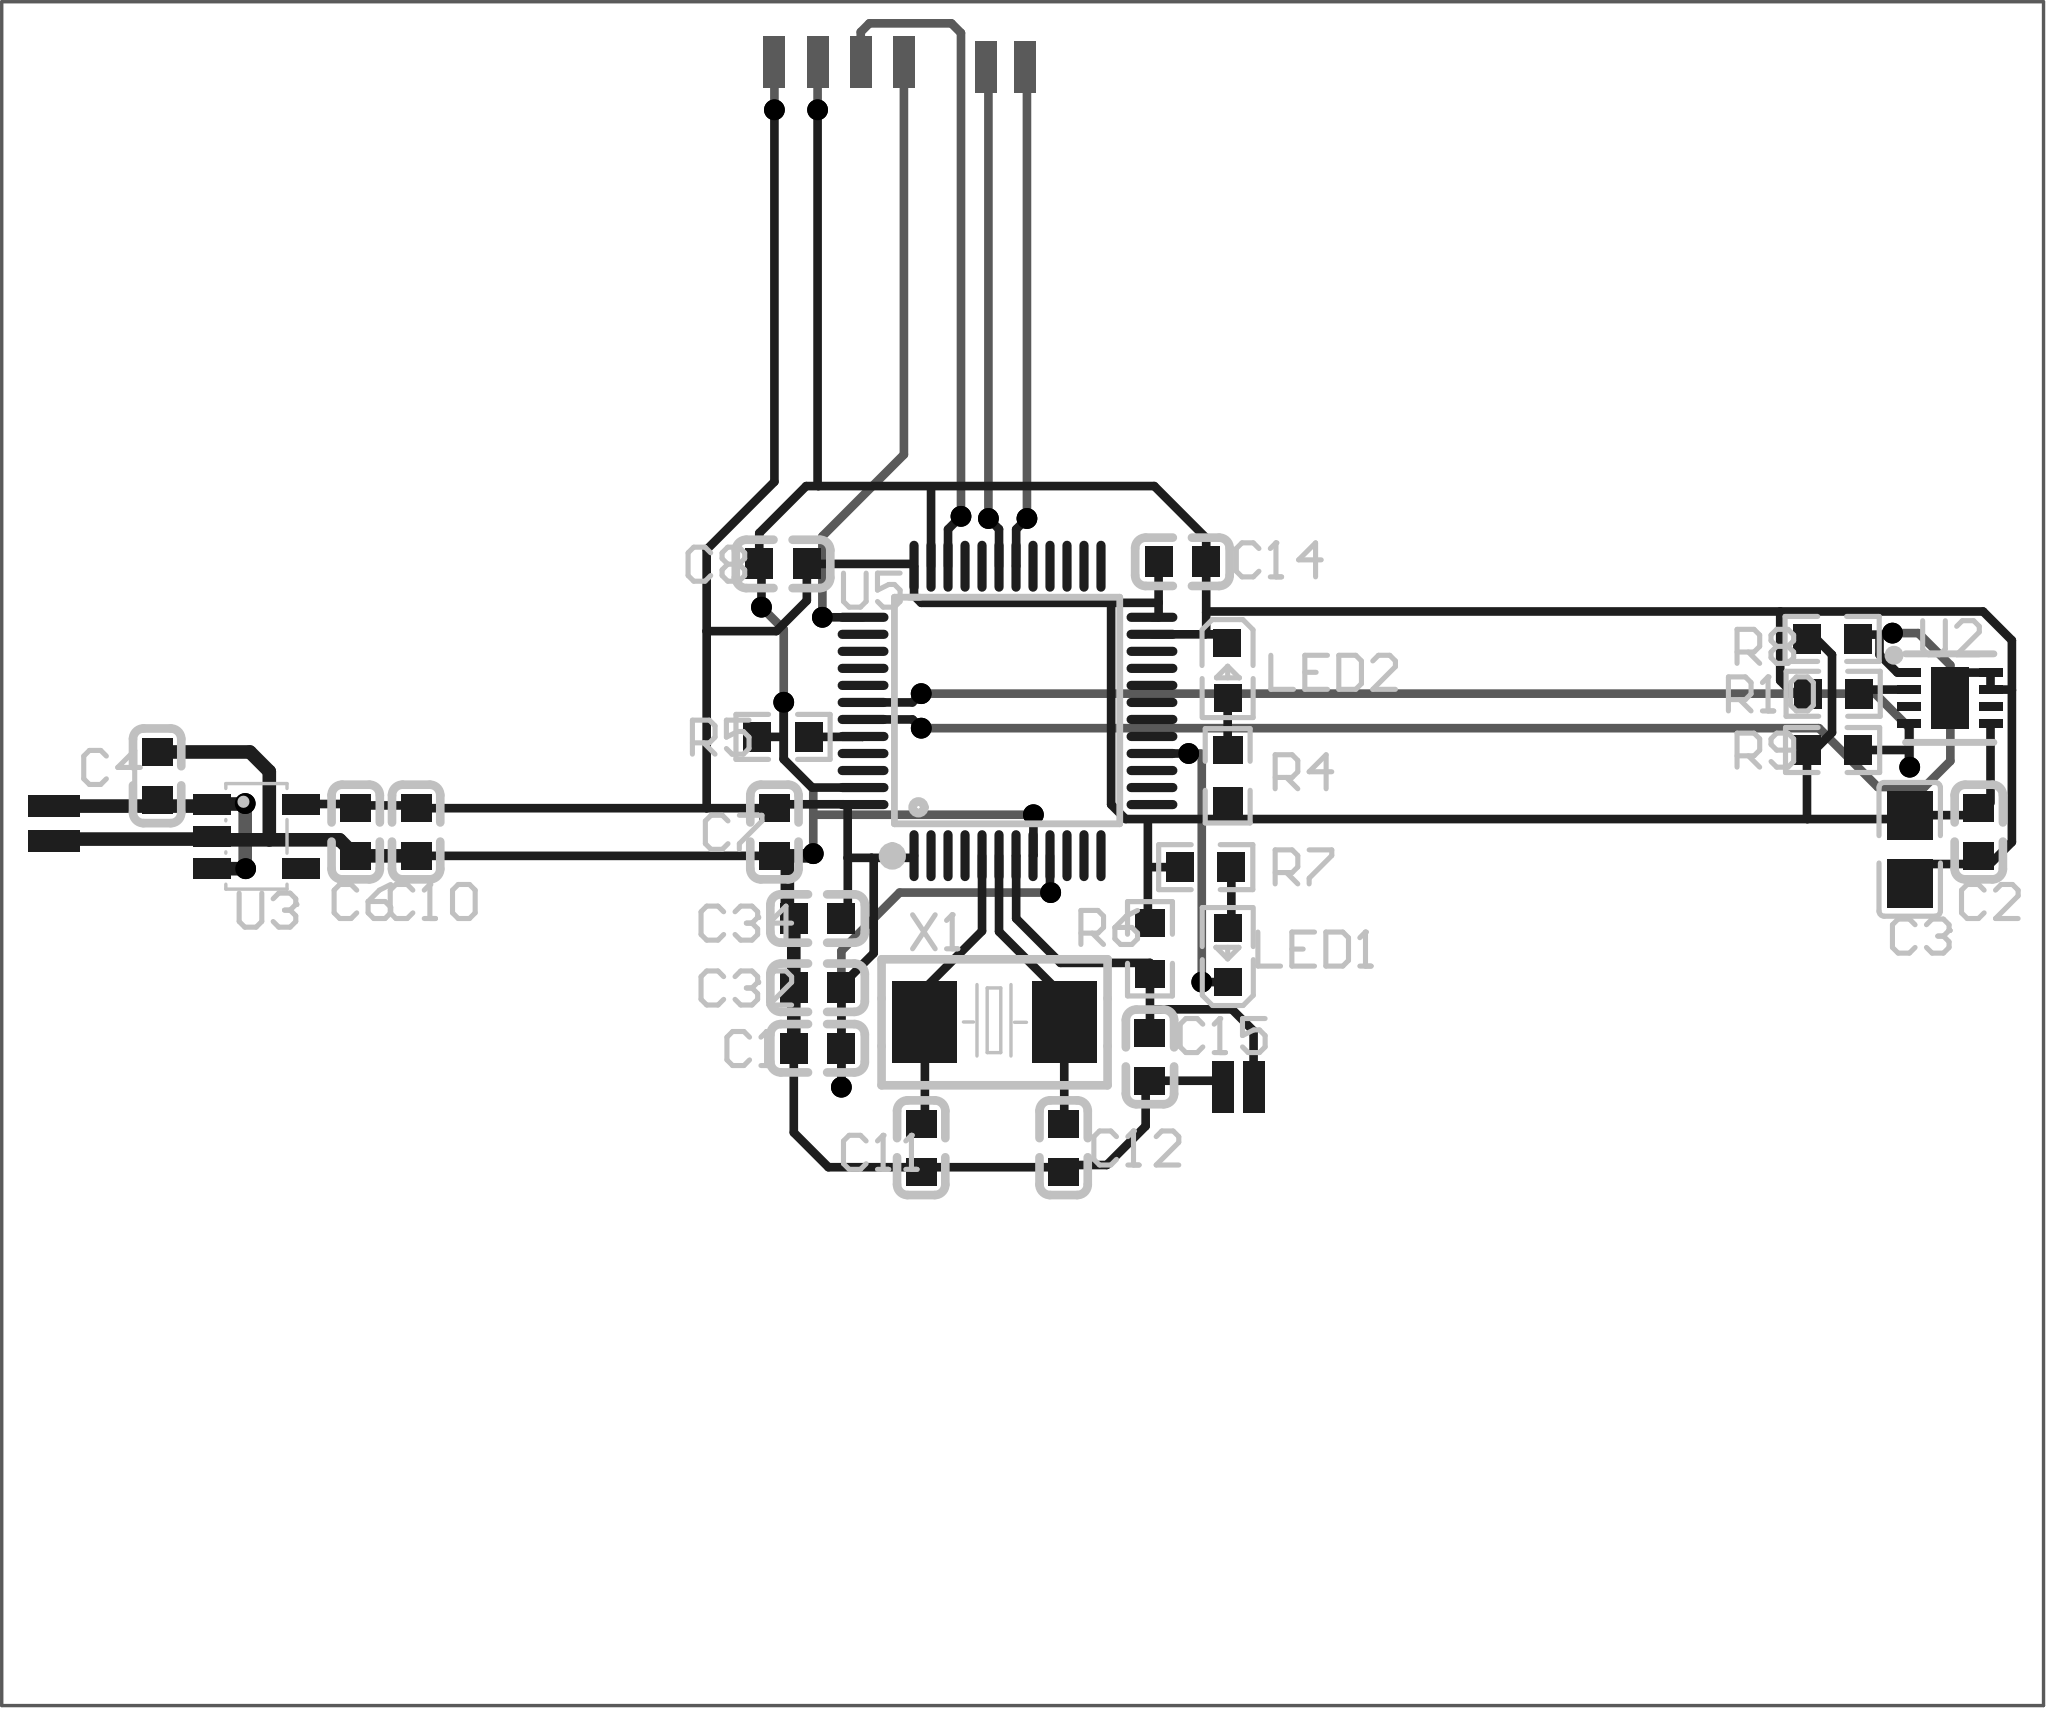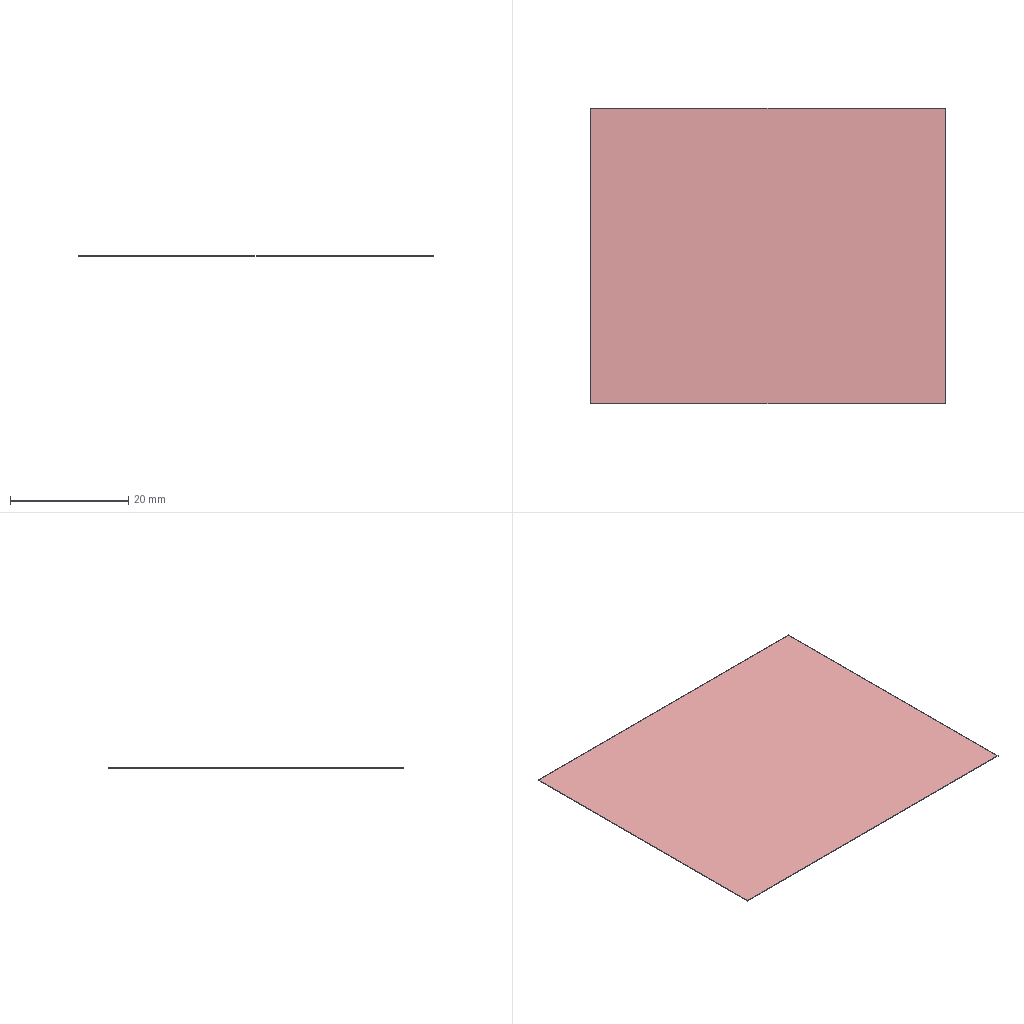Circuit board layout | Altium Designer | box 60.1 x 50 x 0.1 mm
Layer stack:
# Altium Designer layer stack of  (unit mm; dielectric type: 0 none, 1 core, 2 prepreg, 3 surface material)
index,name,kind,layer,copper_thickness_mm,dielectric_type,dielectric_thickness_mm,dielectric_material,dielectric_constant
0,Top Paste Mask Layer,other,,,,,,
1,Top Silkscreen Layer,other,,,,,,
2,Top Solder Mask Layer,dielectric,,,3,0.027,,3.3
3,Top Layer,copper,Top Layer,0.012,,,,
4,Dielectric1,dielectric,,,3,0.025,FR4,4.5
5,Bottom Layer,copper,Bottom Layer,0.012,,,,
6,Bottom Solder Mask Layer,dielectric,,,3,0.027,,3.3
7,Bottom Silkscreen Layer,other,,,,,,
8,Bottom Paste Mask Layer,other,,,,,,
# drill layer pairs: low layer,high layer
drill_pair,Top Layer,Bottom Layer
Part placement:
Designator,Comment,Layer,Footprint,Center-X(mm),Center-Y(mm),Rotation
C7,100nF,TopLayer,C0603,98.933,101.854,90
C8,100nF,TopLayer,C0603,99.187,109.728,180
C14,100nF,TopLayer,C0603,110.936,109.79,0
C15,100nF,TopLayer,C0603,109.982,95.25,270
C32,100nF,TopLayer,C0603,100.203,97.282,0
C34,100nF,TopLayer,C0603,100.203,99.314,180
LED2,,TopLayer,LED_0603,112.26,106.604,270
R4,1K,TopLayer,R0603,112.268,103.505,90
R5,10K,TopLayer,R0603,99.187,104.648,180
R6,10K,TopLayer,R0603,109.982,98.425,90
U5,STM32F103C8T6,TopLayer,LQFP-48_L7.0-W7.0-P0.50-LS9.0-BL,105.791,105.41,0
C2,100nF,TopLayer,C0603,134.366,101.854,270
C3,4.7uF,TopLayer,C0805,132.334,101.346,90
C4,10uF,TopLayer,C0603,80.772,103.505,270
C6,10uF,TopLayer,C0603,86.614,101.854,270
C10,100nF,TopLayer,C0603,88.392,101.854,90
LED1,,TopLayer,LED_0603,112.276,98.247,90
R7,1K,TopLayer,R0603,111.623,100.823,0
R8,10K,TopLayer,R0603,130.052,107.525,180
R9,10K,TopLayer,R0603,130.065,104.263,180
R10,10K,TopLayer,R0603,130.082,105.914,180
U2,SHT30-DIS-B2.5KS,TopLayer,DFN-8_L2.5-W2.5-P0.50-BL-EP,133.511,105.787,270
U3,TLV75533PDBVR,TopLayer,SOT-23-5_L3.0-W1.7-P0.95-LS2.8-BR,83.693,101.727,180
X1,8MHz,TopLayer,CRYSTAL-SMD_L5.0-W3.2,105.41,96.266,180
C11,20pF,TopLayer,C0603,103.251,92.583,90
C12,20pF,TopLayer,C0603,107.442,92.583,90
C1,1uF,TopLayer,C0603,100.203,95.504,0
Pad and via stacks:
# Altium Designer via and pad stacks of  (unit mm). Each distinct definition once, with the count of objects using it.
# via: kind,start_layer,end_layer,hole_mm,diameter_mm,mode(0 simple;1 top-mid-bottom;2 full stack),diameter_per_layer,count,example_net
# pad: kind,layer,hole_mm,hole_type(0 round;1 square;2 slot),plating,top_size,top_shape(1 round;2 rect;3 octagon;9 rounded rect),mid_size,bottom_size,mode,footprint,size_per_layer,count,example
pad,Top Layer,0,0,plated,0.8x0.9,2,0.8x0.9,0.8x0.9,0,C0603,,26,C7.2
pad,Top Layer,0,0,plated,0.8001x0.8001,2,0.8001x0.8001,0.8001x0.8001,0,LED_0603,,4,LED2.1
pad,Top Layer,0,0,plated,0.8065x0.864,2,0.8065x0.864,0.8065x0.864,0,R0603,,14,R4.2
pad,Top Layer,0,0,plated,0.27x1.5,1,0.27x1.5,0.27x1.5,0,LQFP-48_L7.0-W7.0-P0.50-LS9.0-BL,,24,U5.1
pad,Top Layer,0,0,plated,1.5x0.27,1,1.5x0.27,1.5x0.27,0,LQFP-48_L7.0-W7.0-P0.50-LS9.0-BL,,24,U5.13
pad,Top Layer,0,0,plated,1.41x1.35,2,1.41x1.35,1.41x1.35,0,C0805,,2,C3.2
pad,Top Layer,0,0,plated,1.8x1.1,2,1.8x1.1,1.8x1.1,0,DFN-8_L2.5-W2.5-P0.50-BL-EP,,1,U2.9
pad,Top Layer,0,0,plated,0.25x0.7,2,0.25x0.7,0.25x0.7,0,DFN-8_L2.5-W2.5-P0.50-BL-EP,,8,U2.5
pad,Top Layer,0,0,plated,1.1x0.6,2,1.1x0.6,1.1x0.6,0,SOT-23-5_L3.0-W1.7-P0.95-LS2.8-BR,,5,U3.5
pad,Top Layer,0,0,plated,1.524x0.635,2,1.524x0.635,1.524x0.635,0,,,4,4
pad,Top Layer,0,0,plated,1.9x2.4,2,1.9x2.4,1.9x2.4,0,CRYSTAL-SMD_L5.0-W3.2,,2,X1.2
pad,Bottom Layer,0,0,plated,1.524x0.635,2,1.524x0.635,1.524x0.635,0,,,6,1
via,Top Layer,Bottom Layer,0.3048,0.61,0,,20,GND
Design rules, without the lines most boards share:
# Altium Designer design rules of  (exported by Altium Designer, unit mm)
# columns: name | kind | enabled | priority | scope1 | scope2 | descriptor | typed fields (field=value)
HoleToHoleClearance | 52 | enabled | 1 | All | All | Hole To Hole Clearance (Gap=10mil) (All),(All) | gap=0.254
copperThickness1oz | 0 | enabled | 1 | All | All | Clearance Constraint (Gap=7mil) (All),(All) | gap=0.1778
copperThickness1oz_1 | 63 | enabled | 1 | All | All | Board Clearance Constraint (Gap=0mil) (All) |
copperThickness2oz | 0 | enabled | 2 | All | All | Clearance Constraint (Gap=7mil) (All),(All) | gap=0.1778
copperThickness2oz_1 | 63 | enabled | 2 | All | All | Board Clearance Constraint (Gap=0mil) (All) |
otherClearance | 0 | enabled | 3 | All | All | Clearance Constraint (Gap=7mil) (All),(All) | gap=0.1778
otherClearance_1 | 63 | enabled | 3 | All | All | Board Clearance Constraint (Gap=0mil) (All) |
copperThickness1oz_2 | 2 | enabled | 1 | All | All | Width Constraint (Min=5mil) (Max=100mil) (Preferred=10mil) (All) |
copperThickness2oz_2 | 2 | enabled | 2 | All | All | Width Constraint (Min=8mil) (Max=100mil) (Preferred=10mil) (All) |
viaSize | 11 | enabled | 1 | All | All | Routing Via (MinHoleWidth=11.811mil) (MaxHoleWidth=248.031mil) (PreferredHoleWidth=12.008mil) (MinWidth=11.811mil) (MaxWidth=248.031mil) (PreferedWidth=12.008mil) (All) | via_min_hole=0.3 via_max_hole=6.3 via_preferred_diameter=0.305 via_preferred_hole=0.305